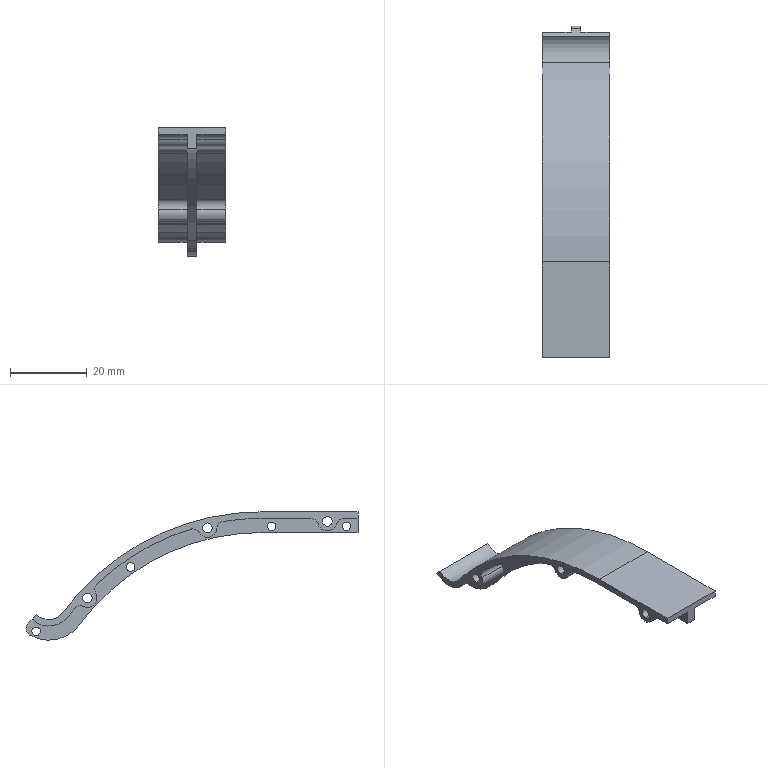Part | SolidWorks | features Extrusion 1, Fillet 1, HoleWzd 1, ICE 1 | 1 solid | 61 faces | box 17.6 x 86.542 x 33.473 mm | volume 4076 mm3 | cylinder 49 | plane 12 | commonest cylinder face diameters 4 x17 2.2 x8 2.5 x6 5 x6 125.6 x6 12.4 x2